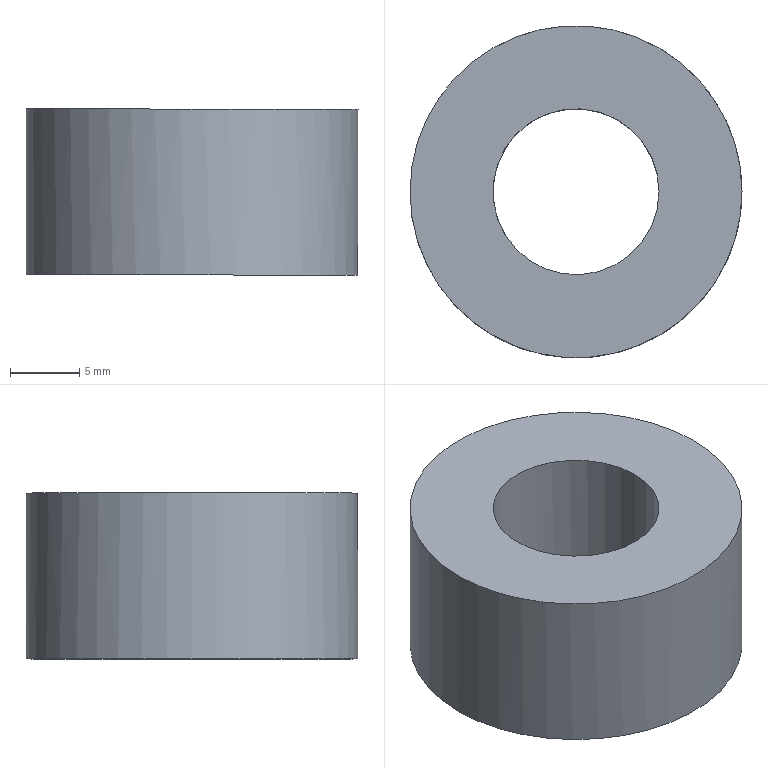Part | NX | features solid 2 | 1 solid | 4 faces | box 24 x 24 x 12 mm | volume 4072 mm3 | plane 2 | cylinder 2 | commonest cylinder face diameters 12 x1 24 x1
STEP:
#1=CARTESIAN_POINT('',(-9.,99.3,5.5));
#2=VERTEX_POINT('',#1);
#3=CARTESIAN_POINT('',(-15.,99.3,5.5));
#4=DIRECTION('',(0.000000009,0.,1.));
#5=DIRECTION('',(1.,0.,-0.000000009));
#6=AXIS2_PLACEMENT_3D('',#3,#4,#5);
#7=CIRCLE('',#6,6.);
#8=EDGE_CURVE('',#2,#2,#7,.T.);
#9=ORIENTED_EDGE('',*,*,#8,.F.);
#10=EDGE_LOOP('',(#9));
#11=FACE_BOUND('',#10,.T.);
#12=CARTESIAN_POINT('',(-3.,99.3,5.5));
#13=VERTEX_POINT('',#12);
#14=CARTESIAN_POINT('',(-15.,99.3,5.5));
#15=DIRECTION('',(0.000000009,0.,1.));
#16=DIRECTION('',(1.,0.,-0.000000009));
#17=AXIS2_PLACEMENT_3D('',#14,#15,#16);
#18=CIRCLE('',#17,12.);
#19=EDGE_CURVE('',#13,#13,#18,.F.);
#20=ORIENTED_EDGE('',*,*,#19,.F.);
#21=EDGE_LOOP('',(#20));
#22=FACE_BOUND('',#21,.T.);
#23=CARTESIAN_POINT('',(-15.,99.3,5.5));
#24=DIRECTION('',(0.000000009,0.,1.));
#25=DIRECTION('',(-1.,0.,0.000000009));
#26=AXIS2_PLACEMENT_3D('',#23,#24,#25);
#27=PLANE('',#26);
#28=ADVANCED_FACE('',(#11,#22),#27,.T.);
#29=CARTESIAN_POINT('',(-21.,99.3,-6.5));
#30=VERTEX_POINT('',#29);
#31=CARTESIAN_POINT('',(-15.,99.3,-6.5));
#32=DIRECTION('',(-0.000000009,0.,-1.));
#33=DIRECTION('',(-1.,0.,0.000000009));
#34=AXIS2_PLACEMENT_3D('',#31,#32,#33);
#35=CIRCLE('',#34,6.);
#36=EDGE_CURVE('',#30,#30,#35,.T.);
#37=ORIENTED_EDGE('',*,*,#36,.F.);
#38=EDGE_LOOP('',(#37));
#39=FACE_BOUND('',#38,.T.);
#40=CARTESIAN_POINT('',(-27.,99.3,-6.5));
#41=VERTEX_POINT('',#40);
#42=CARTESIAN_POINT('',(-15.,99.3,-6.5));
#43=DIRECTION('',(-0.000000009,0.,-1.));
#44=DIRECTION('',(-1.,-0.000000075,0.000000009));
#45=AXIS2_PLACEMENT_3D('',#42,#43,#44);
#46=CIRCLE('',#45,12.);
#47=EDGE_CURVE('',#41,#41,#46,.F.);
#48=ORIENTED_EDGE('',*,*,#47,.F.);
#49=EDGE_LOOP('',(#48));
#50=FACE_BOUND('',#49,.T.);
#51=CARTESIAN_POINT('',(-15.,99.3,-6.5));
#52=DIRECTION('',(-0.000000009,0.,-1.));
#53=DIRECTION('',(1.,0.,-0.000000009));
#54=AXIS2_PLACEMENT_3D('',#51,#52,#53);
#55=PLANE('',#54);
#56=ADVANCED_FACE('',(#39,#50),#55,.T.);
#57=ORIENTED_EDGE('',*,*,#19,.T.);
#58=EDGE_LOOP('',(#57));
#59=FACE_BOUND('',#58,.T.);
#60=ORIENTED_EDGE('',*,*,#47,.T.);
#61=EDGE_LOOP('',(#60));
#62=FACE_BOUND('',#61,.T.);
#63=CARTESIAN_POINT('',(-15.,99.3,-6.5));
#64=DIRECTION('',(0.000000009,0.,1.));
#65=DIRECTION('',(-1.,-0.000000075,0.000000009));
#66=AXIS2_PLACEMENT_3D('',#63,#64,#65);
#67=CYLINDRICAL_SURFACE('',#66,12.);
#68=ADVANCED_FACE('',(#59,#62),#67,.T.);
#69=ORIENTED_EDGE('',*,*,#8,.T.);
#70=EDGE_LOOP('',(#69));
#71=FACE_BOUND('',#70,.T.);
#72=ORIENTED_EDGE('',*,*,#36,.T.);
#73=EDGE_LOOP('',(#72));
#74=FACE_BOUND('',#73,.T.);
#75=CARTESIAN_POINT('',(-15.,99.3,-3.5));
#76=DIRECTION('',(-0.000000009,0.,-1.));
#77=DIRECTION('',(0.,1.,0.));
#78=AXIS2_PLACEMENT_3D('',#75,#76,#77);
#79=CYLINDRICAL_SURFACE('',#78,6.);
#80=ADVANCED_FACE('',(#71,#74),#79,.F.);
#81=CLOSED_SHELL('',(#28,#56,#68,#80));
#82=MANIFOLD_SOLID_BREP('',#81);
#83=(LENGTH_UNIT()NAMED_UNIT(*)SI_UNIT(.MILLI.,.METRE.));
#84=UNCERTAINTY_MEASURE_WITH_UNIT(LENGTH_MEASURE(0.00001),#83,'','');
#85=(NAMED_UNIT(*)PLANE_ANGLE_UNIT()SI_UNIT($,.RADIAN.));
#86=(NAMED_UNIT(*)SI_UNIT($,.STERADIAN.)SOLID_ANGLE_UNIT());
#87=(GEOMETRIC_REPRESENTATION_CONTEXT(3)GLOBAL_UNCERTAINTY_ASSIGNED_CONTEXT((#84))GLOBAL_UNIT_ASSIGNED_CONTEXT((#83,#85,#86))REPRESENTATION_CONTEXT('',''));
#88=ADVANCED_BREP_SHAPE_REPRESENTATION('',(#82),#87);